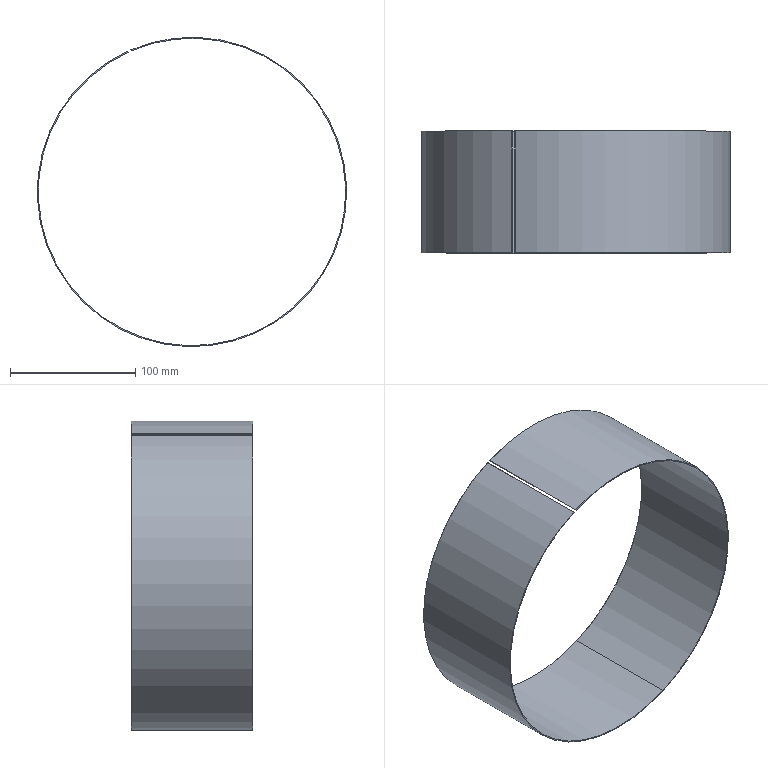Part | STEP file | 1 solid | 8 faces | box 246.568 x 97.02 x 246.568 mm | volume 58546 mm3 | plane 4 | cylinder 4 | commonest cylinder face diameters 245 x2 246.568 x2
STEP:
#1=CARTESIAN_POINT('',(0.,0.,0.));
#2=DIRECTION('',(0.,0.,1.));
#3=DIRECTION('',(1.,0.,0.));
#4=AXIS2_PLACEMENT_3D('',#1,#2,#3);
#5=CARTESIAN_POINT('',(901.591,-52.616,274.274));
#6=VERTEX_POINT('',#5);
#7=CARTESIAN_POINT('',(901.273,-52.616,274.991));
#8=VERTEX_POINT('',#7);
#9=CARTESIAN_POINT('',(900.508,-52.616,276.722));
#10=DIRECTION('',(-0.4047,0.,0.9145));
#11=VECTOR('',#10,1.);
#12=LINE('',#9,#11);
#13=CARTESIAN_POINT('',(900.508,-52.616,276.722));
#14=DIRECTION('',(0.9145,0.,0.4047));
#15=DIRECTION('',(-0.4047,0.,0.9145));
#16=AXIS2_PLACEMENT_3D('',#13,#14,#15);
#17=PLANE('',#16);
#18=CARTESIAN_POINT('',(0.,0.));
#19=DIRECTION('',(1.,0.));
#20=VECTOR('',#19,1.);
#21=LINE('',#18,#20);
#22=(GEOMETRIC_REPRESENTATION_CONTEXT(2)PARAMETRIC_REPRESENTATION_CONTEXT()REPRESENTATION_CONTEXT('',''));
#23=DEFINITIONAL_REPRESENTATION('',(#21),#22);
#24=PCURVE('',#17,#23);
#25=CARTESIAN_POINT('',(950.039,-52.616,161.762));
#26=DIRECTION('',(0.,1.,0.));
#27=DIRECTION('',(0.9145,0.,0.4047));
#28=AXIS2_PLACEMENT_3D('',#25,#26,#27);
#29=PLANE('',#28);
#30=CARTESIAN_POINT('',(1.225,-125.17));
#31=DIRECTION('',(0.,-1.));
#32=VECTOR('',#31,1.);
#33=LINE('',#30,#32);
#34=(GEOMETRIC_REPRESENTATION_CONTEXT(2)PARAMETRIC_REPRESENTATION_CONTEXT()REPRESENTATION_CONTEXT('',''));
#35=DEFINITIONAL_REPRESENTATION('',(#33),#34);
#36=PCURVE('',#29,#35);
#37=SURFACE_CURVE('',#12,(#24,#36),.PCURVE_S1.);
#38=EDGE_CURVE('',#6,#8,#37,.T.);
#39=ORIENTED_EDGE('',*,*,#38,.F.);
#40=CARTESIAN_POINT('',(901.591,-149.636,274.274));
#41=VERTEX_POINT('',#40);
#42=CARTESIAN_POINT('',(901.591,-52.616,274.274));
#43=DIRECTION('',(0.,-1.,0.));
#44=VECTOR('',#43,1.);
#45=LINE('',#42,#44);
#46=CARTESIAN_POINT('',(-2.676,0.));
#47=DIRECTION('',(0.,1.));
#48=VECTOR('',#47,1.);
#49=LINE('',#46,#48);
#50=(GEOMETRIC_REPRESENTATION_CONTEXT(2)PARAMETRIC_REPRESENTATION_CONTEXT()REPRESENTATION_CONTEXT('',''));
#51=DEFINITIONAL_REPRESENTATION('',(#49),#50);
#52=PCURVE('',#17,#51);
#53=CARTESIAN_POINT('',(950.039,-52.616,161.762));
#54=DIRECTION('',(0.,-1.,0.));
#55=DIRECTION('',(0.4047,0.,-0.9145));
#56=AXIS2_PLACEMENT_3D('',#53,#54,#55);
#57=CYLINDRICAL_SURFACE('',#56,122.5);
#58=CARTESIAN_POINT('',(3.132,0.));
#59=DIRECTION('',(0.,1.));
#60=VECTOR('',#59,1.);
#61=LINE('',#58,#60);
#62=(GEOMETRIC_REPRESENTATION_CONTEXT(2)PARAMETRIC_REPRESENTATION_CONTEXT()REPRESENTATION_CONTEXT('',''));
#63=DEFINITIONAL_REPRESENTATION('',(#61),#62);
#64=PCURVE('',#57,#63);
#65=SURFACE_CURVE('',#45,(#52,#64),.PCURVE_S1.);
#66=EDGE_CURVE('',#6,#41,#65,.T.);
#67=ORIENTED_EDGE('',*,*,#66,.T.);
#68=CARTESIAN_POINT('',(901.273,-149.636,274.991));
#69=VERTEX_POINT('',#68);
#70=CARTESIAN_POINT('',(900.508,-149.636,276.722));
#71=DIRECTION('',(-0.4047,0.,0.9145));
#72=VECTOR('',#71,1.);
#73=LINE('',#70,#72);
#74=CARTESIAN_POINT('',(0.,97.02));
#75=DIRECTION('',(1.,0.));
#76=VECTOR('',#75,1.);
#77=LINE('',#74,#76);
#78=(GEOMETRIC_REPRESENTATION_CONTEXT(2)PARAMETRIC_REPRESENTATION_CONTEXT()REPRESENTATION_CONTEXT('',''));
#79=DEFINITIONAL_REPRESENTATION('',(#77),#78);
#80=PCURVE('',#17,#79);
#81=CARTESIAN_POINT('',(950.039,-149.636,161.762));
#82=DIRECTION('',(0.,1.,0.));
#83=DIRECTION('',(0.9145,0.,0.4047));
#84=AXIS2_PLACEMENT_3D('',#81,#82,#83);
#85=PLANE('',#84);
#86=CARTESIAN_POINT('',(1.225,-125.17));
#87=DIRECTION('',(0.,-1.));
#88=VECTOR('',#87,1.);
#89=LINE('',#86,#88);
#90=(GEOMETRIC_REPRESENTATION_CONTEXT(2)PARAMETRIC_REPRESENTATION_CONTEXT()REPRESENTATION_CONTEXT('',''));
#91=DEFINITIONAL_REPRESENTATION('',(#89),#90);
#92=PCURVE('',#85,#91);
#93=SURFACE_CURVE('',#73,(#80,#92),.PCURVE_S1.);
#94=EDGE_CURVE('',#41,#69,#93,.T.);
#95=ORIENTED_EDGE('',*,*,#94,.T.);
#96=CARTESIAN_POINT('',(901.273,-52.616,274.991));
#97=DIRECTION('',(0.,-1.,0.));
#98=VECTOR('',#97,1.);
#99=LINE('',#96,#98);
#100=CARTESIAN_POINT('',(-1.892,0.));
#101=DIRECTION('',(0.,1.));
#102=VECTOR('',#101,1.);
#103=LINE('',#100,#102);
#104=(GEOMETRIC_REPRESENTATION_CONTEXT(2)PARAMETRIC_REPRESENTATION_CONTEXT()REPRESENTATION_CONTEXT('',''));
#105=DEFINITIONAL_REPRESENTATION('',(#103),#104);
#106=PCURVE('',#17,#105);
#107=CARTESIAN_POINT('',(950.039,-52.616,161.762));
#108=DIRECTION('',(0.,-1.,0.));
#109=DIRECTION('',(0.4047,0.,-0.9145));
#110=AXIS2_PLACEMENT_3D('',#107,#108,#109);
#111=CYLINDRICAL_SURFACE('',#110,123.284);
#112=CARTESIAN_POINT('',(3.132,0.));
#113=DIRECTION('',(0.,1.));
#114=VECTOR('',#113,1.);
#115=LINE('',#112,#114);
#116=(GEOMETRIC_REPRESENTATION_CONTEXT(2)PARAMETRIC_REPRESENTATION_CONTEXT()REPRESENTATION_CONTEXT('',''));
#117=DEFINITIONAL_REPRESENTATION('',(#115),#116);
#118=PCURVE('',#111,#117);
#119=SURFACE_CURVE('',#99,(#106,#118),.PCURVE_S1.);
#120=EDGE_CURVE('',#8,#69,#119,.T.);
#121=ORIENTED_EDGE('',*,*,#120,.F.);
#122=EDGE_LOOP('',(#39,#67,#95,#121));
#123=FACE_BOUND('',#122,.T.);
#124=ADVANCED_FACE('',(#123),#17,.F.);
#125=CARTESIAN_POINT('',(899.033,-149.636,274.));
#126=VERTEX_POINT('',#125);
#127=CARTESIAN_POINT('',(899.35,-149.636,273.283));
#128=VERTEX_POINT('',#127);
#129=CARTESIAN_POINT('',(898.267,-149.636,275.73));
#130=DIRECTION('',(0.4047,0.,-0.9145));
#131=VECTOR('',#130,1.);
#132=LINE('',#129,#131);
#133=CARTESIAN_POINT('',(898.267,-52.616,275.73));
#134=DIRECTION('',(-0.9145,0.,-0.4047));
#135=DIRECTION('',(-0.4047,0.,0.9145));
#136=AXIS2_PLACEMENT_3D('',#133,#134,#135);
#137=PLANE('',#136);
#138=CARTESIAN_POINT('',(0.,-97.02));
#139=DIRECTION('',(-1.,0.));
#140=VECTOR('',#139,1.);
#141=LINE('',#138,#140);
#142=(GEOMETRIC_REPRESENTATION_CONTEXT(2)PARAMETRIC_REPRESENTATION_CONTEXT()REPRESENTATION_CONTEXT('',''));
#143=DEFINITIONAL_REPRESENTATION('',(#141),#142);
#144=PCURVE('',#137,#143);
#145=CARTESIAN_POINT('',(-1.225,-125.17));
#146=DIRECTION('',(0.,1.));
#147=VECTOR('',#146,1.);
#148=LINE('',#145,#147);
#149=(GEOMETRIC_REPRESENTATION_CONTEXT(2)PARAMETRIC_REPRESENTATION_CONTEXT()REPRESENTATION_CONTEXT('',''));
#150=DEFINITIONAL_REPRESENTATION('',(#148),#149);
#151=PCURVE('',#85,#150);
#152=SURFACE_CURVE('',#132,(#144,#151),.PCURVE_S1.);
#153=EDGE_CURVE('',#126,#128,#152,.T.);
#154=ORIENTED_EDGE('',*,*,#153,.T.);
#155=CARTESIAN_POINT('',(899.35,-52.616,273.283));
#156=VERTEX_POINT('',#155);
#157=CARTESIAN_POINT('',(899.35,-52.616,273.283));
#158=DIRECTION('',(0.,1.,0.));
#159=VECTOR('',#158,1.);
#160=LINE('',#157,#159);
#161=CARTESIAN_POINT('',(-2.676,0.));
#162=DIRECTION('',(0.,1.));
#163=VECTOR('',#162,1.);
#164=LINE('',#161,#163);
#165=(GEOMETRIC_REPRESENTATION_CONTEXT(2)PARAMETRIC_REPRESENTATION_CONTEXT()REPRESENTATION_CONTEXT('',''));
#166=DEFINITIONAL_REPRESENTATION('',(#164),#165);
#167=PCURVE('',#137,#166);
#168=CARTESIAN_POINT('',(950.039,-52.616,161.762));
#169=DIRECTION('',(0.,-1.,0.));
#170=DIRECTION('',(0.4047,0.,-0.9145));
#171=AXIS2_PLACEMENT_3D('',#168,#169,#170);
#172=CYLINDRICAL_SURFACE('',#171,122.5);
#173=CARTESIAN_POINT('',(3.152,0.));
#174=DIRECTION('',(0.,-1.));
#175=VECTOR('',#174,1.);
#176=LINE('',#173,#175);
#177=(GEOMETRIC_REPRESENTATION_CONTEXT(2)PARAMETRIC_REPRESENTATION_CONTEXT()REPRESENTATION_CONTEXT('',''));
#178=DEFINITIONAL_REPRESENTATION('',(#176),#177);
#179=PCURVE('',#172,#178);
#180=SURFACE_CURVE('',#160,(#167,#179),.PCURVE_S1.);
#181=EDGE_CURVE('',#128,#156,#180,.T.);
#182=ORIENTED_EDGE('',*,*,#181,.T.);
#183=CARTESIAN_POINT('',(899.033,-52.616,274.));
#184=VERTEX_POINT('',#183);
#185=CARTESIAN_POINT('',(898.267,-52.616,275.73));
#186=DIRECTION('',(0.4047,0.,-0.9145));
#187=VECTOR('',#186,1.);
#188=LINE('',#185,#187);
#189=CARTESIAN_POINT('',(0.,0.));
#190=DIRECTION('',(-1.,0.));
#191=VECTOR('',#190,1.);
#192=LINE('',#189,#191);
#193=(GEOMETRIC_REPRESENTATION_CONTEXT(2)PARAMETRIC_REPRESENTATION_CONTEXT()REPRESENTATION_CONTEXT('',''));
#194=DEFINITIONAL_REPRESENTATION('',(#192),#193);
#195=PCURVE('',#137,#194);
#196=CARTESIAN_POINT('',(-1.225,-125.17));
#197=DIRECTION('',(0.,1.));
#198=VECTOR('',#197,1.);
#199=LINE('',#196,#198);
#200=(GEOMETRIC_REPRESENTATION_CONTEXT(2)PARAMETRIC_REPRESENTATION_CONTEXT()REPRESENTATION_CONTEXT('',''));
#201=DEFINITIONAL_REPRESENTATION('',(#199),#200);
#202=PCURVE('',#29,#201);
#203=SURFACE_CURVE('',#188,(#195,#202),.PCURVE_S1.);
#204=EDGE_CURVE('',#184,#156,#203,.T.);
#205=ORIENTED_EDGE('',*,*,#204,.F.);
#206=CARTESIAN_POINT('',(899.033,-52.616,274.));
#207=DIRECTION('',(0.,1.,0.));
#208=VECTOR('',#207,1.);
#209=LINE('',#206,#208);
#210=CARTESIAN_POINT('',(-1.892,0.));
#211=DIRECTION('',(0.,1.));
#212=VECTOR('',#211,1.);
#213=LINE('',#210,#212);
#214=(GEOMETRIC_REPRESENTATION_CONTEXT(2)PARAMETRIC_REPRESENTATION_CONTEXT()REPRESENTATION_CONTEXT('',''));
#215=DEFINITIONAL_REPRESENTATION('',(#213),#214);
#216=PCURVE('',#137,#215);
#217=CARTESIAN_POINT('',(950.039,-52.616,161.762));
#218=DIRECTION('',(0.,-1.,0.));
#219=DIRECTION('',(0.4047,0.,-0.9145));
#220=AXIS2_PLACEMENT_3D('',#217,#218,#219);
#221=CYLINDRICAL_SURFACE('',#220,123.284);
#222=CARTESIAN_POINT('',(3.152,0.));
#223=DIRECTION('',(0.,-1.));
#224=VECTOR('',#223,1.);
#225=LINE('',#222,#224);
#226=(GEOMETRIC_REPRESENTATION_CONTEXT(2)PARAMETRIC_REPRESENTATION_CONTEXT()REPRESENTATION_CONTEXT('',''));
#227=DEFINITIONAL_REPRESENTATION('',(#225),#226);
#228=PCURVE('',#221,#227);
#229=SURFACE_CURVE('',#209,(#216,#228),.PCURVE_S1.);
#230=EDGE_CURVE('',#126,#184,#229,.T.);
#231=ORIENTED_EDGE('',*,*,#230,.F.);
#232=EDGE_LOOP('',(#154,#182,#205,#231));
#233=FACE_BOUND('',#232,.T.);
#234=ADVANCED_FACE('',(#233),#137,.F.);
#235=CARTESIAN_POINT('',(999.61,-149.636,49.74));
#236=VERTEX_POINT('',#235);
#237=CARTESIAN_POINT('',(950.039,-149.636,161.762));
#238=DIRECTION('',(0.,1.,0.));
#239=DIRECTION('',(-0.4047,0.,0.9145));
#240=AXIS2_PLACEMENT_3D('',#237,#238,#239);
#241=CIRCLE('',#240,122.5);
#242=CARTESIAN_POINT('',(9.425,97.02));
#243=DIRECTION('',(-1.,0.));
#244=VECTOR('',#243,1.);
#245=LINE('',#242,#244);
#246=(GEOMETRIC_REPRESENTATION_CONTEXT(2)PARAMETRIC_REPRESENTATION_CONTEXT()REPRESENTATION_CONTEXT('',''));
#247=DEFINITIONAL_REPRESENTATION('',(#245),#246);
#248=PCURVE('',#172,#247);
#249=CARTESIAN_POINT('',(0.,0.));
#250=DIRECTION('',(0.,-1.));
#251=AXIS2_PLACEMENT_2D('',#249,#250);
#252=CIRCLE('',#251,122.5);
#253=(GEOMETRIC_REPRESENTATION_CONTEXT(2)PARAMETRIC_REPRESENTATION_CONTEXT()REPRESENTATION_CONTEXT('',''));
#254=DEFINITIONAL_REPRESENTATION('',(#252),#253);
#255=PCURVE('',#85,#254);
#256=SURFACE_CURVE('',#241,(#248,#255),.PCURVE_S1.);
#257=EDGE_CURVE('',#236,#128,#256,.T.);
#258=ORIENTED_EDGE('',*,*,#257,.T.);
#259=ORIENTED_EDGE('',*,*,#181,.T.);
#260=CARTESIAN_POINT('',(999.61,-52.616,49.74));
#261=VERTEX_POINT('',#260);
#262=CARTESIAN_POINT('',(950.039,-52.616,161.762));
#263=DIRECTION('',(0.,1.,0.));
#264=DIRECTION('',(-0.4047,0.,0.9145));
#265=AXIS2_PLACEMENT_3D('',#262,#263,#264);
#266=CIRCLE('',#265,122.5);
#267=CARTESIAN_POINT('',(9.425,0.));
#268=DIRECTION('',(-1.,0.));
#269=VECTOR('',#268,1.);
#270=LINE('',#267,#269);
#271=(GEOMETRIC_REPRESENTATION_CONTEXT(2)PARAMETRIC_REPRESENTATION_CONTEXT()REPRESENTATION_CONTEXT('',''));
#272=DEFINITIONAL_REPRESENTATION('',(#270),#271);
#273=PCURVE('',#172,#272);
#274=CARTESIAN_POINT('',(0.,0.));
#275=DIRECTION('',(0.,-1.));
#276=AXIS2_PLACEMENT_2D('',#274,#275);
#277=CIRCLE('',#276,122.5);
#278=(GEOMETRIC_REPRESENTATION_CONTEXT(2)PARAMETRIC_REPRESENTATION_CONTEXT()REPRESENTATION_CONTEXT('',''));
#279=DEFINITIONAL_REPRESENTATION('',(#277),#278);
#280=PCURVE('',#29,#279);
#281=SURFACE_CURVE('',#266,(#273,#280),.PCURVE_S1.);
#282=EDGE_CURVE('',#261,#156,#281,.T.);
#283=ORIENTED_EDGE('',*,*,#282,.F.);
#284=CARTESIAN_POINT('',(999.61,-52.616,49.74));
#285=DIRECTION('',(0.,-1.,0.));
#286=VECTOR('',#285,1.);
#287=LINE('',#284,#286);
#288=CARTESIAN_POINT('',(6.283,0.));
#289=DIRECTION('',(0.,1.));
#290=VECTOR('',#289,1.);
#291=LINE('',#288,#290);
#292=(GEOMETRIC_REPRESENTATION_CONTEXT(2)PARAMETRIC_REPRESENTATION_CONTEXT()REPRESENTATION_CONTEXT('',''));
#293=DEFINITIONAL_REPRESENTATION('',(#291),#292);
#294=PCURVE('',#172,#293);
#295=CARTESIAN_POINT('',(0.,0.));
#296=DIRECTION('',(0.,1.));
#297=VECTOR('',#296,1.);
#298=LINE('',#295,#297);
#299=(GEOMETRIC_REPRESENTATION_CONTEXT(2)PARAMETRIC_REPRESENTATION_CONTEXT()REPRESENTATION_CONTEXT('',''));
#300=DEFINITIONAL_REPRESENTATION('',(#298),#299);
#301=PCURVE('',#57,#300);
#302=SURFACE_CURVE('',#287,(#294,#301),.PCURVE_S1.);
#303=EDGE_CURVE('',#261,#236,#302,.T.);
#304=ORIENTED_EDGE('',*,*,#303,.T.);
#305=EDGE_LOOP('',(#258,#259,#283,#304));
#306=FACE_BOUND('',#305,.F.);
#307=ADVANCED_FACE('',(#306),#172,.F.);
#308=CARTESIAN_POINT('',(999.928,-149.636,49.023));
#309=VERTEX_POINT('',#308);
#310=CARTESIAN_POINT('',(950.039,-149.636,161.762));
#311=DIRECTION('',(0.,1.,0.));
#312=DIRECTION('',(-0.4047,0.,0.9145));
#313=AXIS2_PLACEMENT_3D('',#310,#311,#312);
#314=CIRCLE('',#313,123.284);
#315=CARTESIAN_POINT('',(0.,0.));
#316=DIRECTION('',(0.,-1.));
#317=AXIS2_PLACEMENT_2D('',#315,#316);
#318=CIRCLE('',#317,123.284);
#319=(GEOMETRIC_REPRESENTATION_CONTEXT(2)PARAMETRIC_REPRESENTATION_CONTEXT()REPRESENTATION_CONTEXT('',''));
#320=DEFINITIONAL_REPRESENTATION('',(#318),#319);
#321=PCURVE('',#85,#320);
#322=CARTESIAN_POINT('',(3.142,97.02));
#323=DIRECTION('',(-1.,0.));
#324=VECTOR('',#323,1.);
#325=LINE('',#322,#324);
#326=(GEOMETRIC_REPRESENTATION_CONTEXT(2)PARAMETRIC_REPRESENTATION_CONTEXT()REPRESENTATION_CONTEXT('',''));
#327=DEFINITIONAL_REPRESENTATION('',(#325),#326);
#328=PCURVE('',#111,#327);
#329=SURFACE_CURVE('',#314,(#321,#328),.PCURVE_S1.);
#330=EDGE_CURVE('',#69,#309,#329,.T.);
#331=ORIENTED_EDGE('',*,*,#330,.F.);
#332=ORIENTED_EDGE('',*,*,#94,.F.);
#333=CARTESIAN_POINT('',(950.039,-149.636,161.762));
#334=DIRECTION('',(0.,1.,0.));
#335=DIRECTION('',(-0.4047,0.,0.9145));
#336=AXIS2_PLACEMENT_3D('',#333,#334,#335);
#337=CIRCLE('',#336,122.5);
#338=CARTESIAN_POINT('',(0.,0.));
#339=DIRECTION('',(0.,-1.));
#340=AXIS2_PLACEMENT_2D('',#338,#339);
#341=CIRCLE('',#340,122.5);
#342=(GEOMETRIC_REPRESENTATION_CONTEXT(2)PARAMETRIC_REPRESENTATION_CONTEXT()REPRESENTATION_CONTEXT('',''));
#343=DEFINITIONAL_REPRESENTATION('',(#341),#342);
#344=PCURVE('',#85,#343);
#345=CARTESIAN_POINT('',(3.142,97.02));
#346=DIRECTION('',(-1.,0.));
#347=VECTOR('',#346,1.);
#348=LINE('',#345,#347);
#349=(GEOMETRIC_REPRESENTATION_CONTEXT(2)PARAMETRIC_REPRESENTATION_CONTEXT()REPRESENTATION_CONTEXT('',''));
#350=DEFINITIONAL_REPRESENTATION('',(#348),#349);
#351=PCURVE('',#57,#350);
#352=SURFACE_CURVE('',#337,(#344,#351),.PCURVE_S1.);
#353=EDGE_CURVE('',#41,#236,#352,.T.);
#354=ORIENTED_EDGE('',*,*,#353,.T.);
#355=ORIENTED_EDGE('',*,*,#257,.T.);
#356=ORIENTED_EDGE('',*,*,#153,.F.);
#357=CARTESIAN_POINT('',(950.039,-149.636,161.762));
#358=DIRECTION('',(0.,1.,0.));
#359=DIRECTION('',(-0.4047,0.,0.9145));
#360=AXIS2_PLACEMENT_3D('',#357,#358,#359);
#361=CIRCLE('',#360,123.284);
#362=CARTESIAN_POINT('',(0.,0.));
#363=DIRECTION('',(0.,-1.));
#364=AXIS2_PLACEMENT_2D('',#362,#363);
#365=CIRCLE('',#364,123.284);
#366=(GEOMETRIC_REPRESENTATION_CONTEXT(2)PARAMETRIC_REPRESENTATION_CONTEXT()REPRESENTATION_CONTEXT('',''));
#367=DEFINITIONAL_REPRESENTATION('',(#365),#366);
#368=PCURVE('',#85,#367);
#369=CARTESIAN_POINT('',(9.425,97.02));
#370=DIRECTION('',(-1.,0.));
#371=VECTOR('',#370,1.);
#372=LINE('',#369,#371);
#373=(GEOMETRIC_REPRESENTATION_CONTEXT(2)PARAMETRIC_REPRESENTATION_CONTEXT()REPRESENTATION_CONTEXT('',''));
#374=DEFINITIONAL_REPRESENTATION('',(#372),#373);
#375=PCURVE('',#221,#374);
#376=SURFACE_CURVE('',#361,(#368,#375),.PCURVE_S1.);
#377=EDGE_CURVE('',#309,#126,#376,.T.);
#378=ORIENTED_EDGE('',*,*,#377,.F.);
#379=EDGE_LOOP('',(#331,#332,#354,#355,#356,#378));
#380=FACE_BOUND('',#379,.T.);
#381=ADVANCED_FACE('',(#380),#85,.F.);
#382=ORIENTED_EDGE('',*,*,#38,.T.);
#383=CARTESIAN_POINT('',(999.928,-52.616,49.023));
#384=VERTEX_POINT('',#383);
#385=CARTESIAN_POINT('',(950.039,-52.616,161.762));
#386=DIRECTION('',(0.,1.,0.));
#387=DIRECTION('',(-0.4047,0.,0.9145));
#388=AXIS2_PLACEMENT_3D('',#385,#386,#387);
#389=CIRCLE('',#388,123.284);
#390=CARTESIAN_POINT('',(0.,0.));
#391=DIRECTION('',(0.,-1.));
#392=AXIS2_PLACEMENT_2D('',#390,#391);
#393=CIRCLE('',#392,123.284);
#394=(GEOMETRIC_REPRESENTATION_CONTEXT(2)PARAMETRIC_REPRESENTATION_CONTEXT()REPRESENTATION_CONTEXT('',''));
#395=DEFINITIONAL_REPRESENTATION('',(#393),#394);
#396=PCURVE('',#29,#395);
#397=CARTESIAN_POINT('',(3.142,0.));
#398=DIRECTION('',(-1.,0.));
#399=VECTOR('',#398,1.);
#400=LINE('',#397,#399);
#401=(GEOMETRIC_REPRESENTATION_CONTEXT(2)PARAMETRIC_REPRESENTATION_CONTEXT()REPRESENTATION_CONTEXT('',''));
#402=DEFINITIONAL_REPRESENTATION('',(#400),#401);
#403=PCURVE('',#111,#402);
#404=SURFACE_CURVE('',#389,(#396,#403),.PCURVE_S1.);
#405=EDGE_CURVE('',#8,#384,#404,.T.);
#406=ORIENTED_EDGE('',*,*,#405,.T.);
#407=CARTESIAN_POINT('',(950.039,-52.616,161.762));
#408=DIRECTION('',(0.,1.,0.));
#409=DIRECTION('',(-0.4047,0.,0.9145));
#410=AXIS2_PLACEMENT_3D('',#407,#408,#409);
#411=CIRCLE('',#410,123.284);
#412=CARTESIAN_POINT('',(0.,0.));
#413=DIRECTION('',(0.,-1.));
#414=AXIS2_PLACEMENT_2D('',#412,#413);
#415=CIRCLE('',#414,123.284);
#416=(GEOMETRIC_REPRESENTATION_CONTEXT(2)PARAMETRIC_REPRESENTATION_CONTEXT()REPRESENTATION_CONTEXT('',''));
#417=DEFINITIONAL_REPRESENTATION('',(#415),#416);
#418=PCURVE('',#29,#417);
#419=CARTESIAN_POINT('',(9.425,0.));
#420=DIRECTION('',(-1.,0.));
#421=VECTOR('',#420,1.);
#422=LINE('',#419,#421);
#423=(GEOMETRIC_REPRESENTATION_CONTEXT(2)PARAMETRIC_REPRESENTATION_CONTEXT()REPRESENTATION_CONTEXT('',''));
#424=DEFINITIONAL_REPRESENTATION('',(#422),#423);
#425=PCURVE('',#221,#424);
#426=SURFACE_CURVE('',#411,(#418,#425),.PCURVE_S1.);
#427=EDGE_CURVE('',#384,#184,#426,.T.);
#428=ORIENTED_EDGE('',*,*,#427,.T.);
#429=ORIENTED_EDGE('',*,*,#204,.T.);
#430=ORIENTED_EDGE('',*,*,#282,.F.);
#431=CARTESIAN_POINT('',(950.039,-52.616,161.762));
#432=DIRECTION('',(0.,1.,0.));
#433=DIRECTION('',(-0.4047,0.,0.9145));
#434=AXIS2_PLACEMENT_3D('',#431,#432,#433);
#435=CIRCLE('',#434,122.5);
#436=CARTESIAN_POINT('',(0.,0.));
#437=DIRECTION('',(0.,-1.));
#438=AXIS2_PLACEMENT_2D('',#436,#437);
#439=CIRCLE('',#438,122.5);
#440=(GEOMETRIC_REPRESENTATION_CONTEXT(2)PARAMETRIC_REPRESENTATION_CONTEXT()REPRESENTATION_CONTEXT('',''));
#441=DEFINITIONAL_REPRESENTATION('',(#439),#440);
#442=PCURVE('',#29,#441);
#443=CARTESIAN_POINT('',(3.142,0.));
#444=DIRECTION('',(-1.,0.));
#445=VECTOR('',#444,1.);
#446=LINE('',#443,#445);
#447=(GEOMETRIC_REPRESENTATION_CONTEXT(2)PARAMETRIC_REPRESENTATION_CONTEXT()REPRESENTATION_CONTEXT('',''));
#448=DEFINITIONAL_REPRESENTATION('',(#446),#447);
#449=PCURVE('',#57,#448);
#450=SURFACE_CURVE('',#435,(#442,#449),.PCURVE_S1.);
#451=EDGE_CURVE('',#6,#261,#450,.T.);
#452=ORIENTED_EDGE('',*,*,#451,.F.);
#453=EDGE_LOOP('',(#382,#406,#428,#429,#430,#452));
#454=FACE_BOUND('',#453,.T.);
#455=ADVANCED_FACE('',(#454),#29,.T.);
#456=CARTESIAN_POINT('',(999.928,-52.616,49.023));
#457=DIRECTION('',(0.,-1.,0.));
#458=VECTOR('',#457,1.);
#459=LINE('',#456,#458);
#460=CARTESIAN_POINT('',(0.,0.));
#461=DIRECTION('',(0.,1.));
#462=VECTOR('',#461,1.);
#463=LINE('',#460,#462);
#464=(GEOMETRIC_REPRESENTATION_CONTEXT(2)PARAMETRIC_REPRESENTATION_CONTEXT()REPRESENTATION_CONTEXT('',''));
#465=DEFINITIONAL_REPRESENTATION('',(#463),#464);
#466=PCURVE('',#111,#465);
#467=CARTESIAN_POINT('',(6.283,0.));
#468=DIRECTION('',(0.,1.));
#469=VECTOR('',#468,1.);
#470=LINE('',#467,#469);
#471=(GEOMETRIC_REPRESENTATION_CONTEXT(2)PARAMETRIC_REPRESENTATION_CONTEXT()REPRESENTATION_CONTEXT('',''));
#472=DEFINITIONAL_REPRESENTATION('',(#470),#471);
#473=PCURVE('',#221,#472);
#474=SURFACE_CURVE('',#459,(#466,#473),.PCURVE_S1.);
#475=EDGE_CURVE('',#384,#309,#474,.T.);
#476=ORIENTED_EDGE('',*,*,#475,.F.);
#477=ORIENTED_EDGE('',*,*,#405,.F.);
#478=ORIENTED_EDGE('',*,*,#120,.T.);
#479=ORIENTED_EDGE('',*,*,#330,.T.);
#480=EDGE_LOOP('',(#476,#477,#478,#479));
#481=FACE_BOUND('',#480,.T.);
#482=ADVANCED_FACE('',(#481),#111,.T.);
#483=ORIENTED_EDGE('',*,*,#427,.F.);
#484=ORIENTED_EDGE('',*,*,#475,.T.);
#485=ORIENTED_EDGE('',*,*,#377,.T.);
#486=ORIENTED_EDGE('',*,*,#230,.T.);
#487=EDGE_LOOP('',(#483,#484,#485,#486));
#488=FACE_BOUND('',#487,.T.);
#489=ADVANCED_FACE('',(#488),#221,.T.);
#490=ORIENTED_EDGE('',*,*,#66,.T.);
#491=ORIENTED_EDGE('',*,*,#353,.T.);
#492=ORIENTED_EDGE('',*,*,#303,.F.);
#493=ORIENTED_EDGE('',*,*,#451,.F.);
#494=EDGE_LOOP('',(#490,#491,#492,#493));
#495=FACE_BOUND('',#494,.F.);
#496=ADVANCED_FACE('',(#495),#57,.F.);
#497=CLOSED_SHELL('',(#124,#234,#307,#381,#455,#482,#489,#496));
#498=MANIFOLD_SOLID_BREP('',#497);
#499=(LENGTH_UNIT()NAMED_UNIT(*)SI_UNIT(.MILLI.,.METRE.));
#500=UNCERTAINTY_MEASURE_WITH_UNIT(LENGTH_MEASURE(0.0000001),#499,'','');
#501=(NAMED_UNIT(*)PLANE_ANGLE_UNIT()SI_UNIT($,.RADIAN.));
#502=(NAMED_UNIT(*)SI_UNIT($,.STERADIAN.)SOLID_ANGLE_UNIT());
#503=(GEOMETRIC_REPRESENTATION_CONTEXT(3)GLOBAL_UNCERTAINTY_ASSIGNED_CONTEXT((#500))GLOBAL_UNIT_ASSIGNED_CONTEXT((#499,#501,#502))REPRESENTATION_CONTEXT('',''));
#504=ADVANCED_BREP_SHAPE_REPRESENTATION('',(#4,#498),#503);